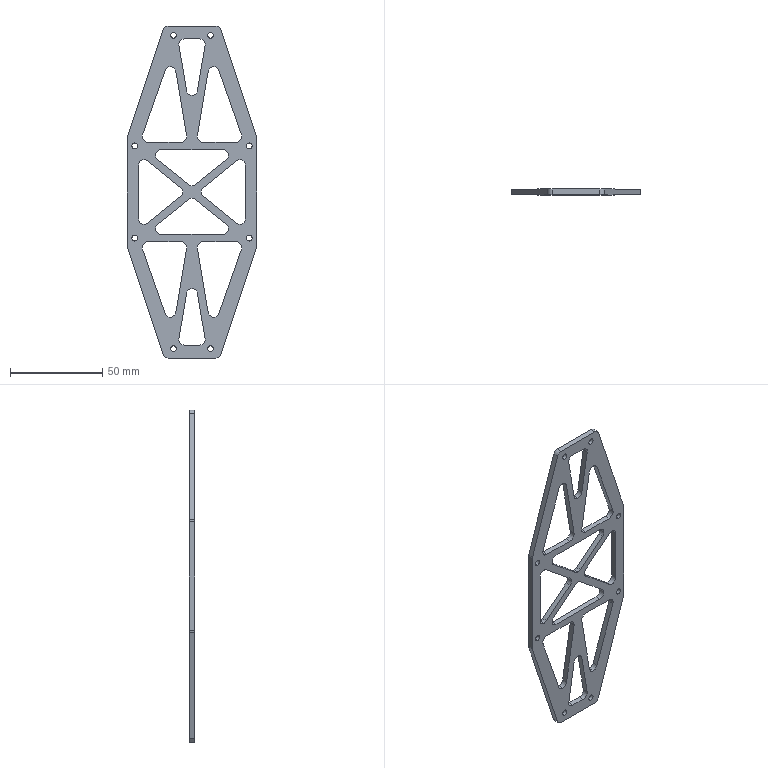Part | SolidWorks | features ICE 2, Extrusion 1, Fillet 1 | 1 solid | 100 faces | box 70 x 3 x 180 mm | volume 15170 mm3 | cylinder 60 | plane 40 | commonest cylinder face diameters 6 x44 3.2 x16